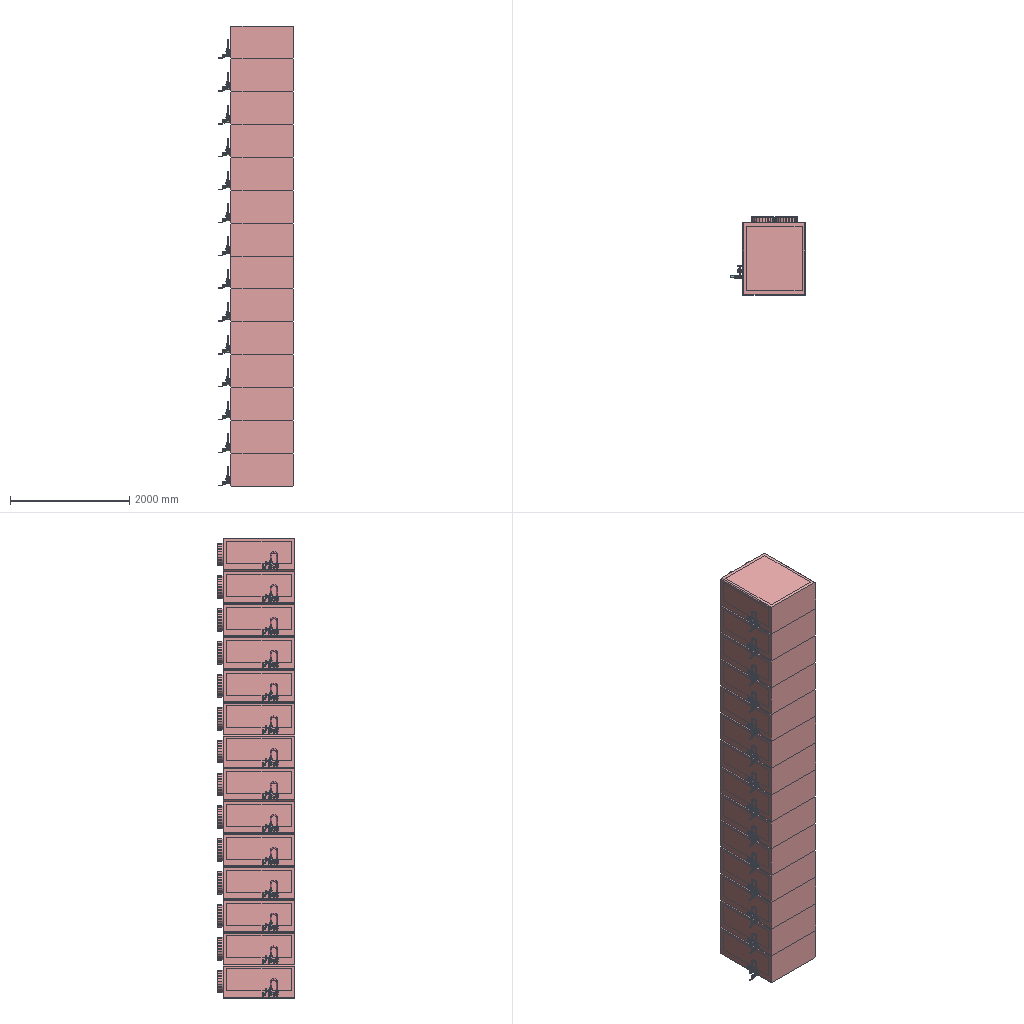Assembly | SolidWorks | 8 different items | 140 placed | box 1261 x 1300 x 7703 mm
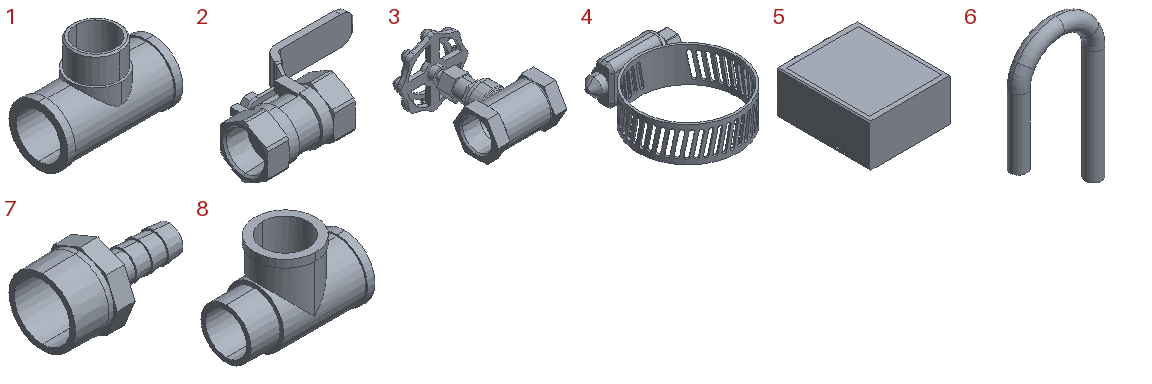Parts list (item | quantity | size | volume | features):
1 | x14 | 78 x 40 x 59 mm | 38405 mm3 | features ICE 2, Revolution 2, Chamfer 1
2 | x14 | 136 x 70.001 x 42.56 mm | 63816 mm3 | features BaseBody 3
3 | x14 | 72 x 115.407 x 70 mm | 83947 mm3 | features BaseBody 1
4 | x28 | 23 x 29.251 x 9 mm | 732.821 mm3 | features ICE 7, Chamfer 2, Fillet 2, CirPattern 1, ExtruThin 1
5 | x14 | 1080 x 1300 x 550.2 mm | 708299280 mm3 | features ICE 14, LPattern 2, Chamfer 1, CirPattern 1, Extrusion 1, Fillet 1, HoleWzd 1
6 | x14 | 122 x 22 x 210.99 mm | 81123 mm3 | features Sweep 1
7 | x28 | 64 x 37.343 x 37.343 mm | 11465 mm3 | features ICE 1, Revolution 1
8 | x14 | 78 x 40 x 57 mm | 38567 mm3 | features ICE 2, Revolution 2, Chamfer 1
Mates (type | each side: item.copy, entity, surface, feature):
Concentric | 5.1 face cone Boss-Extrude2 | 1.1 face cylinder Revolve1
DistanceDim | 5.1 face plane Boss-Extrude3 | 1.1 face plane Revolve1
Concentric | 5.1 face cone Boss-Extrude2 | 8.1 face cylinder Revolve1
DistanceDim | 8.1 face plane Revolve1 | 5.1 face plane Boss-Extrude3
Concentric | 8.1 face cylinder Revolve1 | 2.1 face cone BSFFA25A_b.stp-1-solid1
DistanceDim | 2.1 face plane BSFFA25A_b.stp-1-solid1 | 8.1 face plane Revolve1
Concentric | 1.1 face cylinder Revolve2 | 3.1 face cone Input1
DistanceDim | 3.1 face plane Input1 | 1.1 face plane Revolve2
Concentric | 3.1 face cone Input1 | 7.1 face cone Revolve1
Coincident | 3.1 face plane Input1 | 7.1 edge
Concentric | 8.1 face cylinder Revolve2 | 7.2 face cone Revolve1
Coincident | 8.1 face plane Revolve2 | 7.2 edge
Parallel | 5.1 face plane Boss-Extrude1 | 3.1 face plane Input1
Concentric | 7.1 face cylinder Revolve1 | 6.1 face cylinder Sweep1
DistanceDim | 6.1 face plane Sweep1 | 7.1 face plane Revolve1
Parallel | 5.1 face plane Boss-Extrude1 | 8.1 face plane Revolve2
Concentric | 6.1 face cylinder Sweep1 | 4.1 face cylinder Extrude-Thin1
Coincident | 6.1 face plane Sweep1 | 4.1 face plane Extrude-Thin1
Concentric | 6.1 face cylinder Sweep1 | 4.2 face cylinder Extrude-Thin1
Coincident | 6.1 face plane Sweep1 | 4.2 face plane Extrude-Thin1